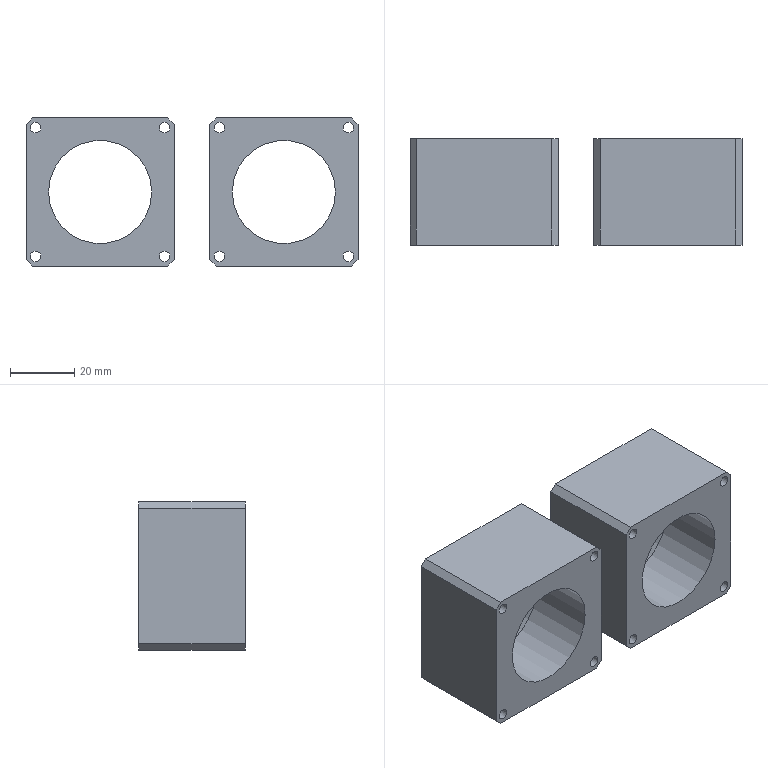Part | 2 solids | 74 faces | box 103 x 33 x 46 mm | volume 71791 mm3 | plane 38 | cylinder 30 | cone 6 | commonest cylinder face diameters 3.3 x8 4 x8 2.5 x6 39 x6 32 x2